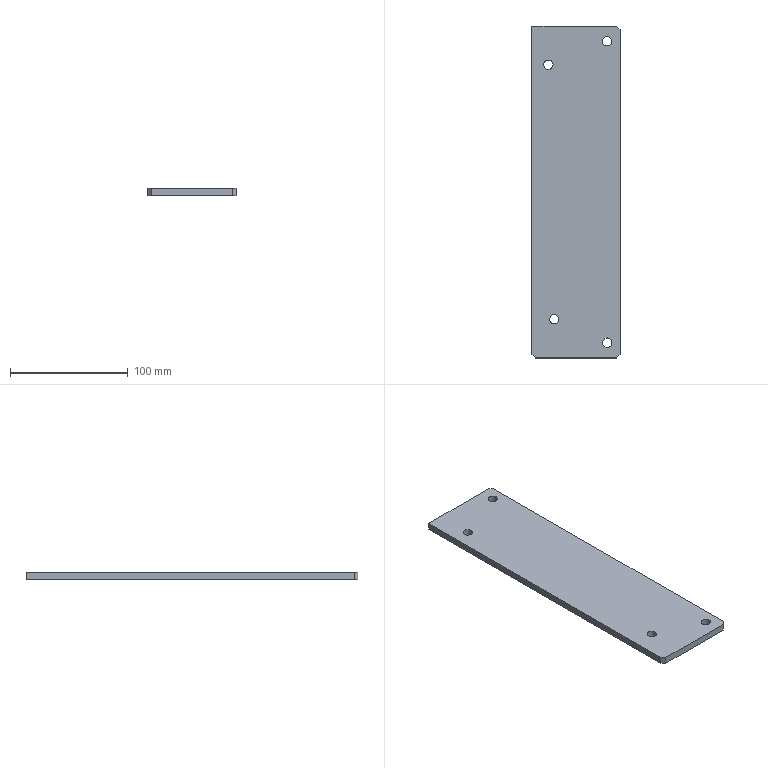Part | STEP file | 1_id1326_x_t | 1 solid | 13 faces | box 75 x 282.347 x 6 mm | volume 125769 mm3 | plane 9 | cylinder 4 | commonest cylinder face diameters 8 x4
STEP:
#1=CARTESIAN_POINT('',(0.,0.,0.));
#2=DIRECTION('',(0.,0.,1.));
#3=DIRECTION('',(1.,0.,0.));
#4=AXIS2_PLACEMENT_3D('',#1,#2,#3);
#5=CARTESIAN_POINT('',(-8.,318.523,-6.));
#6=VERTEX_POINT('',#5);
#7=CARTESIAN_POINT('',(-80.,318.523,-6.));
#8=VERTEX_POINT('',#7);
#9=CARTESIAN_POINT('',(-8.,318.523,-6.));
#10=DIRECTION('',(-1.,0.,0.));
#11=VECTOR('',#10,1.);
#12=LINE('',#9,#11);
#13=CARTESIAN_POINT('',(-80.,-0.15,-6.));
#14=DIRECTION('',(0.,0.,-1.));
#15=DIRECTION('',(-1.,0.,0.));
#16=AXIS2_PLACEMENT_3D('',#13,#14,#15);
#17=PLANE('',#16);
#18=CARTESIAN_POINT('',(-72.,318.673));
#19=DIRECTION('',(1.,0.));
#20=VECTOR('',#19,1.);
#21=LINE('',#18,#20);
#22=(GEOMETRIC_REPRESENTATION_CONTEXT(2)PARAMETRIC_REPRESENTATION_CONTEXT()REPRESENTATION_CONTEXT('',''));
#23=DEFINITIONAL_REPRESENTATION('',(#21),#22);
#24=PCURVE('',#17,#23);
#25=CARTESIAN_POINT('',(669.363,318.523,-130.047));
#26=DIRECTION('',(0.,1.,0.));
#27=DIRECTION('',(-1.,0.,0.));
#28=AXIS2_PLACEMENT_3D('',#25,#26,#27);
#29=PLANE('',#28);
#30=CARTESIAN_POINT('',(677.363,124.047));
#31=DIRECTION('',(1.,0.));
#32=VECTOR('',#31,1.);
#33=LINE('',#30,#32);
#34=(GEOMETRIC_REPRESENTATION_CONTEXT(2)PARAMETRIC_REPRESENTATION_CONTEXT()REPRESENTATION_CONTEXT('',''));
#35=DEFINITIONAL_REPRESENTATION('',(#33),#34);
#36=PCURVE('',#29,#35);
#37=SURFACE_CURVE('',#12,(#24,#36),.PCURVE_S1.);
#38=EDGE_CURVE('',#6,#8,#37,.T.);
#39=ORIENTED_EDGE('',*,*,#38,.F.);
#40=CARTESIAN_POINT('',(-5.,315.523,-6.));
#41=VERTEX_POINT('',#40);
#42=CARTESIAN_POINT('',(-8.,318.523,-6.));
#43=DIRECTION('',(0.7071,-0.7071,0.));
#44=VECTOR('',#43,1.);
#45=LINE('',#42,#44);
#46=CARTESIAN_POINT('',(-72.,318.673));
#47=DIRECTION('',(-0.7071,-0.7071));
#48=VECTOR('',#47,1.);
#49=LINE('',#46,#48);
#50=(GEOMETRIC_REPRESENTATION_CONTEXT(2)PARAMETRIC_REPRESENTATION_CONTEXT()REPRESENTATION_CONTEXT('',''));
#51=DEFINITIONAL_REPRESENTATION('',(#49),#50);
#52=PCURVE('',#17,#51);
#53=CARTESIAN_POINT('',(-8.,318.523,-130.047));
#54=DIRECTION('',(0.7071,0.7071,0.));
#55=DIRECTION('',(-0.7071,0.7071,0.));
#56=AXIS2_PLACEMENT_3D('',#53,#54,#55);
#57=PLANE('',#56);
#58=CARTESIAN_POINT('',(0.,124.047));
#59=DIRECTION('',(-1.,0.));
#60=VECTOR('',#59,1.);
#61=LINE('',#58,#60);
#62=(GEOMETRIC_REPRESENTATION_CONTEXT(2)PARAMETRIC_REPRESENTATION_CONTEXT()REPRESENTATION_CONTEXT('',''));
#63=DEFINITIONAL_REPRESENTATION('',(#61),#62);
#64=PCURVE('',#57,#63);
#65=SURFACE_CURVE('',#45,(#52,#64),.PCURVE_S1.);
#66=EDGE_CURVE('',#6,#41,#65,.T.);
#67=ORIENTED_EDGE('',*,*,#66,.T.);
#68=CARTESIAN_POINT('',(-5.,39.177,-6.));
#69=VERTEX_POINT('',#68);
#70=CARTESIAN_POINT('',(-5.,315.523,-6.));
#71=DIRECTION('',(0.,-1.,0.));
#72=VECTOR('',#71,1.);
#73=LINE('',#70,#72);
#74=CARTESIAN_POINT('',(-75.,315.673));
#75=DIRECTION('',(0.,-1.));
#76=VECTOR('',#75,1.);
#77=LINE('',#74,#76);
#78=(GEOMETRIC_REPRESENTATION_CONTEXT(2)PARAMETRIC_REPRESENTATION_CONTEXT()REPRESENTATION_CONTEXT('',''));
#79=DEFINITIONAL_REPRESENTATION('',(#77),#78);
#80=PCURVE('',#17,#79);
#81=CARTESIAN_POINT('',(-5.,-0.15,0.));
#82=DIRECTION('',(-1.,0.,0.));
#83=DIRECTION('',(0.,-1.,0.));
#84=AXIS2_PLACEMENT_3D('',#81,#82,#83);
#85=PLANE('',#84);
#86=CARTESIAN_POINT('',(-315.673,-6.));
#87=DIRECTION('',(1.,0.));
#88=VECTOR('',#87,1.);
#89=LINE('',#86,#88);
#90=(GEOMETRIC_REPRESENTATION_CONTEXT(2)PARAMETRIC_REPRESENTATION_CONTEXT()REPRESENTATION_CONTEXT('',''));
#91=DEFINITIONAL_REPRESENTATION('',(#89),#90);
#92=PCURVE('',#85,#91);
#93=SURFACE_CURVE('',#73,(#80,#92),.PCURVE_S1.);
#94=EDGE_CURVE('',#41,#69,#93,.T.);
#95=ORIENTED_EDGE('',*,*,#94,.T.);
#96=CARTESIAN_POINT('',(-8.,36.177,-6.));
#97=VERTEX_POINT('',#96);
#98=CARTESIAN_POINT('',(-5.,39.177,-6.));
#99=DIRECTION('',(-0.7071,-0.7071,0.));
#100=VECTOR('',#99,1.);
#101=LINE('',#98,#100);
#102=CARTESIAN_POINT('',(-75.,39.327));
#103=DIRECTION('',(0.7071,-0.7071));
#104=VECTOR('',#103,1.);
#105=LINE('',#102,#104);
#106=(GEOMETRIC_REPRESENTATION_CONTEXT(2)PARAMETRIC_REPRESENTATION_CONTEXT()REPRESENTATION_CONTEXT('',''));
#107=DEFINITIONAL_REPRESENTATION('',(#105),#106);
#108=PCURVE('',#17,#107);
#109=CARTESIAN_POINT('',(-5.,39.177,0.));
#110=DIRECTION('',(0.7071,-0.7071,0.));
#111=DIRECTION('',(0.7071,0.7071,0.));
#112=AXIS2_PLACEMENT_3D('',#109,#110,#111);
#113=PLANE('',#112);
#114=CARTESIAN_POINT('',(0.,-6.));
#115=DIRECTION('',(-1.,0.));
#116=VECTOR('',#115,1.);
#117=LINE('',#114,#116);
#118=(GEOMETRIC_REPRESENTATION_CONTEXT(2)PARAMETRIC_REPRESENTATION_CONTEXT()REPRESENTATION_CONTEXT('',''));
#119=DEFINITIONAL_REPRESENTATION('',(#117),#118);
#120=PCURVE('',#113,#119);
#121=SURFACE_CURVE('',#101,(#108,#120),.PCURVE_S1.);
#122=EDGE_CURVE('',#69,#97,#121,.T.);
#123=ORIENTED_EDGE('',*,*,#122,.T.);
#124=CARTESIAN_POINT('',(-77.,36.177,-6.));
#125=VERTEX_POINT('',#124);
#126=CARTESIAN_POINT('',(-8.,36.177,-6.));
#127=DIRECTION('',(-1.,0.,0.));
#128=VECTOR('',#127,1.);
#129=LINE('',#126,#128);
#130=CARTESIAN_POINT('',(-72.,36.327));
#131=DIRECTION('',(1.,0.));
#132=VECTOR('',#131,1.);
#133=LINE('',#130,#132);
#134=(GEOMETRIC_REPRESENTATION_CONTEXT(2)PARAMETRIC_REPRESENTATION_CONTEXT()REPRESENTATION_CONTEXT('',''));
#135=DEFINITIONAL_REPRESENTATION('',(#133),#134);
#136=PCURVE('',#17,#135);
#137=CARTESIAN_POINT('',(661.363,36.177,-130.047));
#138=DIRECTION('',(0.,-1.,0.));
#139=DIRECTION('',(-1.,0.,0.));
#140=AXIS2_PLACEMENT_3D('',#137,#138,#139);
#141=PLANE('',#140);
#142=CARTESIAN_POINT('',(669.363,-124.047));
#143=DIRECTION('',(1.,0.));
#144=VECTOR('',#143,1.);
#145=LINE('',#142,#144);
#146=(GEOMETRIC_REPRESENTATION_CONTEXT(2)PARAMETRIC_REPRESENTATION_CONTEXT()REPRESENTATION_CONTEXT('',''));
#147=DEFINITIONAL_REPRESENTATION('',(#145),#146);
#148=PCURVE('',#141,#147);
#149=SURFACE_CURVE('',#129,(#136,#148),.PCURVE_S1.);
#150=EDGE_CURVE('',#97,#125,#149,.T.);
#151=ORIENTED_EDGE('',*,*,#150,.T.);
#152=CARTESIAN_POINT('',(-80.,39.177,-6.));
#153=VERTEX_POINT('',#152);
#154=CARTESIAN_POINT('',(-77.,36.177,-6.));
#155=DIRECTION('',(-0.7071,0.7071,0.));
#156=VECTOR('',#155,1.);
#157=LINE('',#154,#156);
#158=CARTESIAN_POINT('',(-3.,36.327));
#159=DIRECTION('',(0.7071,0.7071));
#160=VECTOR('',#159,1.);
#161=LINE('',#158,#160);
#162=(GEOMETRIC_REPRESENTATION_CONTEXT(2)PARAMETRIC_REPRESENTATION_CONTEXT()REPRESENTATION_CONTEXT('',''));
#163=DEFINITIONAL_REPRESENTATION('',(#161),#162);
#164=PCURVE('',#17,#163);
#165=CARTESIAN_POINT('',(-77.,36.177,-130.047));
#166=DIRECTION('',(0.7071,0.7071,0.));
#167=DIRECTION('',(-0.7071,0.7071,0.));
#168=AXIS2_PLACEMENT_3D('',#165,#166,#167);
#169=PLANE('',#168);
#170=CARTESIAN_POINT('',(0.,124.047));
#171=DIRECTION('',(1.,0.));
#172=VECTOR('',#171,1.);
#173=LINE('',#170,#172);
#174=(GEOMETRIC_REPRESENTATION_CONTEXT(2)PARAMETRIC_REPRESENTATION_CONTEXT()REPRESENTATION_CONTEXT('',''));
#175=DEFINITIONAL_REPRESENTATION('',(#173),#174);
#176=PCURVE('',#169,#175);
#177=SURFACE_CURVE('',#157,(#164,#176),.PCURVE_S1.);
#178=EDGE_CURVE('',#125,#153,#177,.T.);
#179=ORIENTED_EDGE('',*,*,#178,.T.);
#180=CARTESIAN_POINT('',(-80.,318.523,-6.));
#181=DIRECTION('',(0.,-1.,0.));
#182=VECTOR('',#181,1.);
#183=LINE('',#180,#182);
#184=CARTESIAN_POINT('',(0.,318.673));
#185=DIRECTION('',(0.,-1.));
#186=VECTOR('',#185,1.);
#187=LINE('',#184,#186);
#188=(GEOMETRIC_REPRESENTATION_CONTEXT(2)PARAMETRIC_REPRESENTATION_CONTEXT()REPRESENTATION_CONTEXT('',''));
#189=DEFINITIONAL_REPRESENTATION('',(#187),#188);
#190=PCURVE('',#17,#189);
#191=CARTESIAN_POINT('',(-80.,-0.15,0.));
#192=DIRECTION('',(-1.,0.,0.));
#193=DIRECTION('',(0.,-1.,0.));
#194=AXIS2_PLACEMENT_3D('',#191,#192,#193);
#195=PLANE('',#194);
#196=CARTESIAN_POINT('',(-318.673,-6.));
#197=DIRECTION('',(1.,0.));
#198=VECTOR('',#197,1.);
#199=LINE('',#196,#198);
#200=(GEOMETRIC_REPRESENTATION_CONTEXT(2)PARAMETRIC_REPRESENTATION_CONTEXT()REPRESENTATION_CONTEXT('',''));
#201=DEFINITIONAL_REPRESENTATION('',(#199),#200);
#202=PCURVE('',#195,#201);
#203=SURFACE_CURVE('',#183,(#190,#202),.PCURVE_S1.);
#204=EDGE_CURVE('',#8,#153,#203,.T.);
#205=ORIENTED_EDGE('',*,*,#204,.F.);
#206=EDGE_LOOP('',(#39,#67,#95,#123,#151,#179,#205));
#207=FACE_BOUND('',#206,.T.);
#208=CARTESIAN_POINT('',(-16.,45.177,-6.));
#209=VERTEX_POINT('',#208);
#210=CARTESIAN_POINT('',(-16.,53.177,-6.));
#211=VERTEX_POINT('',#210);
#212=CARTESIAN_POINT('',(-16.,49.177,-6.));
#213=DIRECTION('',(0.,0.,1.));
#214=DIRECTION('',(0.,-1.,0.));
#215=AXIS2_PLACEMENT_3D('',#212,#213,#214);
#216=CIRCLE('',#215,4.);
#217=CARTESIAN_POINT('',(-64.,45.327));
#218=CARTESIAN_POINT('',(-70.928,45.327));
#219=CARTESIAN_POINT('',(-67.464,51.327));
#220=CARTESIAN_POINT('',(-64.,57.327));
#221=CARTESIAN_POINT('',(-60.536,51.327));
#222=CARTESIAN_POINT('',(-57.072,45.327));
#223=CARTESIAN_POINT('',(-64.,45.327));
#224=(BOUNDED_CURVE()B_SPLINE_CURVE(2,(#217,#218,#219,#220,#221,#222,#223),.UNSPECIFIED.,.T.,.F.)B_SPLINE_CURVE_WITH_KNOTS((1,2,2,2,2,1),(-2.094,0.,2.094,4.189,6.283,8.378),.UNSPECIFIED.)CURVE()GEOMETRIC_REPRESENTATION_ITEM()RATIONAL_B_SPLINE_CURVE((1.,0.5,1.,0.5,1.,0.5,1.))REPRESENTATION_ITEM(''));
#225=(GEOMETRIC_REPRESENTATION_CONTEXT(2)PARAMETRIC_REPRESENTATION_CONTEXT()REPRESENTATION_CONTEXT('',''));
#226=DEFINITIONAL_REPRESENTATION('',(#224),#225);
#227=PCURVE('',#17,#226);
#228=CARTESIAN_POINT('',(-16.,49.177,-6.));
#229=DIRECTION('',(0.,0.,1.));
#230=DIRECTION('',(0.,1.,0.));
#231=AXIS2_PLACEMENT_3D('',#228,#229,#230);
#232=CYLINDRICAL_SURFACE('',#231,4.);
#233=CARTESIAN_POINT('',(3.142,0.));
#234=DIRECTION('',(1.,0.));
#235=VECTOR('',#234,1.);
#236=LINE('',#233,#235);
#237=(GEOMETRIC_REPRESENTATION_CONTEXT(2)PARAMETRIC_REPRESENTATION_CONTEXT()REPRESENTATION_CONTEXT('',''));
#238=DEFINITIONAL_REPRESENTATION('',(#236),#237);
#239=PCURVE('',#232,#238);
#240=SURFACE_CURVE('',#216,(#227,#239),.PCURVE_S1.);
#241=EDGE_CURVE('',#209,#211,#240,.T.);
#242=ORIENTED_EDGE('',*,*,#241,.T.);
#243=CARTESIAN_POINT('',(-16.,49.177,-6.));
#244=DIRECTION('',(0.,0.,1.));
#245=DIRECTION('',(0.,-1.,0.));
#246=AXIS2_PLACEMENT_3D('',#243,#244,#245);
#247=CIRCLE('',#246,4.);
#248=CARTESIAN_POINT('',(-64.,45.327));
#249=CARTESIAN_POINT('',(-70.928,45.327));
#250=CARTESIAN_POINT('',(-67.464,51.327));
#251=CARTESIAN_POINT('',(-64.,57.327));
#252=CARTESIAN_POINT('',(-60.536,51.327));
#253=CARTESIAN_POINT('',(-57.072,45.327));
#254=CARTESIAN_POINT('',(-64.,45.327));
#255=(BOUNDED_CURVE()B_SPLINE_CURVE(2,(#248,#249,#250,#251,#252,#253,#254),.UNSPECIFIED.,.T.,.F.)B_SPLINE_CURVE_WITH_KNOTS((1,2,2,2,2,1),(-2.094,0.,2.094,4.189,6.283,8.378),.UNSPECIFIED.)CURVE()GEOMETRIC_REPRESENTATION_ITEM()RATIONAL_B_SPLINE_CURVE((1.,0.5,1.,0.5,1.,0.5,1.))REPRESENTATION_ITEM(''));
#256=(GEOMETRIC_REPRESENTATION_CONTEXT(2)PARAMETRIC_REPRESENTATION_CONTEXT()REPRESENTATION_CONTEXT('',''));
#257=DEFINITIONAL_REPRESENTATION('',(#255),#256);
#258=PCURVE('',#17,#257);
#259=CARTESIAN_POINT('',(-3.142,0.));
#260=DIRECTION('',(1.,0.));
#261=VECTOR('',#260,1.);
#262=LINE('',#259,#261);
#263=(GEOMETRIC_REPRESENTATION_CONTEXT(2)PARAMETRIC_REPRESENTATION_CONTEXT()REPRESENTATION_CONTEXT('',''));
#264=DEFINITIONAL_REPRESENTATION('',(#262),#263);
#265=PCURVE('',#232,#264);
#266=SURFACE_CURVE('',#247,(#258,#265),.PCURVE_S1.);
#267=EDGE_CURVE('',#211,#209,#266,.T.);
#268=ORIENTED_EDGE('',*,*,#267,.T.);
#269=EDGE_LOOP('',(#242,#268));
#270=FACE_BOUND('',#269,.T.);
#271=CARTESIAN_POINT('',(-61.,65.177,-6.));
#272=VERTEX_POINT('',#271);
#273=CARTESIAN_POINT('',(-57.,69.177,-6.));
#274=VERTEX_POINT('',#273);
#275=CARTESIAN_POINT('',(-61.,69.177,-6.));
#276=DIRECTION('',(0.,0.,1.));
#277=DIRECTION('',(0.,-1.,0.));
#278=AXIS2_PLACEMENT_3D('',#275,#276,#277);
#279=CIRCLE('',#278,4.);
#280=CARTESIAN_POINT('',(-19.,65.327));
#281=CARTESIAN_POINT('',(-25.928,65.327));
#282=CARTESIAN_POINT('',(-22.464,71.327));
#283=CARTESIAN_POINT('',(-19.,77.327));
#284=CARTESIAN_POINT('',(-15.536,71.327));
#285=CARTESIAN_POINT('',(-12.072,65.327));
#286=CARTESIAN_POINT('',(-19.,65.327));
#287=(BOUNDED_CURVE()B_SPLINE_CURVE(2,(#280,#281,#282,#283,#284,#285,#286),.UNSPECIFIED.,.T.,.F.)B_SPLINE_CURVE_WITH_KNOTS((1,2,2,2,2,1),(-2.094,0.,2.094,4.189,6.283,8.378),.UNSPECIFIED.)CURVE()GEOMETRIC_REPRESENTATION_ITEM()RATIONAL_B_SPLINE_CURVE((1.,0.5,1.,0.5,1.,0.5,1.))REPRESENTATION_ITEM(''));
#288=(GEOMETRIC_REPRESENTATION_CONTEXT(2)PARAMETRIC_REPRESENTATION_CONTEXT()REPRESENTATION_CONTEXT('',''));
#289=DEFINITIONAL_REPRESENTATION('',(#287),#288);
#290=PCURVE('',#17,#289);
#291=CARTESIAN_POINT('',(-61.,69.177,-6.));
#292=DIRECTION('',(0.,0.,1.));
#293=DIRECTION('',(0.,1.,0.));
#294=AXIS2_PLACEMENT_3D('',#291,#292,#293);
#295=CYLINDRICAL_SURFACE('',#294,4.);
#296=CARTESIAN_POINT('',(9.425,0.));
#297=DIRECTION('',(1.,0.));
#298=VECTOR('',#297,1.);
#299=LINE('',#296,#298);
#300=(GEOMETRIC_REPRESENTATION_CONTEXT(2)PARAMETRIC_REPRESENTATION_CONTEXT()REPRESENTATION_CONTEXT('',''));
#301=DEFINITIONAL_REPRESENTATION('',(#299),#300);
#302=PCURVE('',#295,#301);
#303=SURFACE_CURVE('',#279,(#290,#302),.PCURVE_S1.);
#304=EDGE_CURVE('',#272,#274,#303,.T.);
#305=ORIENTED_EDGE('',*,*,#304,.T.);
#306=CARTESIAN_POINT('',(-61.,69.177,-6.));
#307=DIRECTION('',(0.,0.,1.));
#308=DIRECTION('',(0.,-1.,0.));
#309=AXIS2_PLACEMENT_3D('',#306,#307,#308);
#310=CIRCLE('',#309,4.);
#311=CARTESIAN_POINT('',(-19.,65.327));
#312=CARTESIAN_POINT('',(-25.928,65.327));
#313=CARTESIAN_POINT('',(-22.464,71.327));
#314=CARTESIAN_POINT('',(-19.,77.327));
#315=CARTESIAN_POINT('',(-15.536,71.327));
#316=CARTESIAN_POINT('',(-12.072,65.327));
#317=CARTESIAN_POINT('',(-19.,65.327));
#318=(BOUNDED_CURVE()B_SPLINE_CURVE(2,(#311,#312,#313,#314,#315,#316,#317),.UNSPECIFIED.,.T.,.F.)B_SPLINE_CURVE_WITH_KNOTS((1,2,2,2,2,1),(-2.094,0.,2.094,4.189,6.283,8.378),.UNSPECIFIED.)CURVE()GEOMETRIC_REPRESENTATION_ITEM()RATIONAL_B_SPLINE_CURVE((1.,0.5,1.,0.5,1.,0.5,1.))REPRESENTATION_ITEM(''));
#319=(GEOMETRIC_REPRESENTATION_CONTEXT(2)PARAMETRIC_REPRESENTATION_CONTEXT()REPRESENTATION_CONTEXT('',''));
#320=DEFINITIONAL_REPRESENTATION('',(#318),#319);
#321=PCURVE('',#17,#320);
#322=CARTESIAN_POINT('',(3.142,0.));
#323=DIRECTION('',(1.,0.));
#324=VECTOR('',#323,1.);
#325=LINE('',#322,#324);
#326=(GEOMETRIC_REPRESENTATION_CONTEXT(2)PARAMETRIC_REPRESENTATION_CONTEXT()REPRESENTATION_CONTEXT('',''));
#327=DEFINITIONAL_REPRESENTATION('',(#325),#326);
#328=PCURVE('',#295,#327);
#329=SURFACE_CURVE('',#310,(#321,#328),.PCURVE_S1.);
#330=EDGE_CURVE('',#274,#272,#329,.T.);
#331=ORIENTED_EDGE('',*,*,#330,.T.);
#332=EDGE_LOOP('',(#305,#331));
#333=FACE_BOUND('',#332,.T.);
#334=CARTESIAN_POINT('',(-66.,289.523,-6.));
#335=VERTEX_POINT('',#334);
#336=CARTESIAN_POINT('',(-62.,285.523,-6.));
#337=VERTEX_POINT('',#336);
#338=CARTESIAN_POINT('',(-66.,285.523,-6.));
#339=DIRECTION('',(0.,0.,1.));
#340=DIRECTION('',(0.,1.,0.));
#341=AXIS2_PLACEMENT_3D('',#338,#339,#340);
#342=CIRCLE('',#341,4.);
#343=CARTESIAN_POINT('',(-14.,289.673));
#344=CARTESIAN_POINT('',(-7.072,289.673));
#345=CARTESIAN_POINT('',(-10.536,283.673));
#346=CARTESIAN_POINT('',(-14.,277.673));
#347=CARTESIAN_POINT('',(-17.464,283.673));
#348=CARTESIAN_POINT('',(-20.928,289.673));
#349=CARTESIAN_POINT('',(-14.,289.673));
#350=(BOUNDED_CURVE()B_SPLINE_CURVE(2,(#343,#344,#345,#346,#347,#348,#349),.UNSPECIFIED.,.T.,.F.)B_SPLINE_CURVE_WITH_KNOTS((1,2,2,2,2,1),(-2.094,0.,2.094,4.189,6.283,8.378),.UNSPECIFIED.)CURVE()GEOMETRIC_REPRESENTATION_ITEM()RATIONAL_B_SPLINE_CURVE((1.,0.5,1.,0.5,1.,0.5,1.))REPRESENTATION_ITEM(''));
#351=(GEOMETRIC_REPRESENTATION_CONTEXT(2)PARAMETRIC_REPRESENTATION_CONTEXT()REPRESENTATION_CONTEXT('',''));
#352=DEFINITIONAL_REPRESENTATION('',(#350),#351);
#353=PCURVE('',#17,#352);
#354=CARTESIAN_POINT('',(-66.,285.523,-6.));
#355=DIRECTION('',(0.,0.,1.));
#356=DIRECTION('',(0.,-1.,0.));
#357=AXIS2_PLACEMENT_3D('',#354,#355,#356);
#358=CYLINDRICAL_SURFACE('',#357,4.);
#359=CARTESIAN_POINT('',(3.142,0.));
#360=DIRECTION('',(1.,0.));
#361=VECTOR('',#360,1.);
#362=LINE('',#359,#361);
#363=(GEOMETRIC_REPRESENTATION_CONTEXT(2)PARAMETRIC_REPRESENTATION_CONTEXT()REPRESENTATION_CONTEXT('',''));
#364=DEFINITIONAL_REPRESENTATION('',(#362),#363);
#365=PCURVE('',#358,#364);
#366=SURFACE_CURVE('',#342,(#353,#365),.PCURVE_S1.);
#367=EDGE_CURVE('',#335,#337,#366,.T.);
#368=ORIENTED_EDGE('',*,*,#367,.T.);
#369=CARTESIAN_POINT('',(-66.,285.523,-6.));
#370=DIRECTION('',(0.,0.,1.));
#371=DIRECTION('',(0.,1.,0.));
#372=AXIS2_PLACEMENT_3D('',#369,#370,#371);
#373=CIRCLE('',#372,4.);
#374=CARTESIAN_POINT('',(-14.,289.673));
#375=CARTESIAN_POINT('',(-7.072,289.673));
#376=CARTESIAN_POINT('',(-10.536,283.673));
#377=CARTESIAN_POINT('',(-14.,277.673));
#378=CARTESIAN_POINT('',(-17.464,283.673));
#379=CARTESIAN_POINT('',(-20.928,289.673));
#380=CARTESIAN_POINT('',(-14.,289.673));
#381=(BOUNDED_CURVE()B_SPLINE_CURVE(2,(#374,#375,#376,#377,#378,#379,#380),.UNSPECIFIED.,.T.,.F.)B_SPLINE_CURVE_WITH_KNOTS((1,2,2,2,2,1),(-2.094,0.,2.094,4.189,6.283,8.378),.UNSPECIFIED.)CURVE()GEOMETRIC_REPRESENTATION_ITEM()RATIONAL_B_SPLINE_CURVE((1.,0.5,1.,0.5,1.,0.5,1.))REPRESENTATION_ITEM(''));
#382=(GEOMETRIC_REPRESENTATION_CONTEXT(2)PARAMETRIC_REPRESENTATION_CONTEXT()REPRESENTATION_CONTEXT('',''));
#383=DEFINITIONAL_REPRESENTATION('',(#381),#382);
#384=PCURVE('',#17,#383);
#385=CARTESIAN_POINT('',(-3.142,0.));
#386=DIRECTION('',(1.,0.));
#387=VECTOR('',#386,1.);
#388=LINE('',#385,#387);
#389=(GEOMETRIC_REPRESENTATION_CONTEXT(2)PARAMETRIC_REPRESENTATION_CONTEXT()REPRESENTATION_CONTEXT('',''));
#390=DEFINITIONAL_REPRESENTATION('',(#388),#389);
#391=PCURVE('',#358,#390);
#392=SURFACE_CURVE('',#373,(#384,#391),.PCURVE_S1.);
#393=EDGE_CURVE('',#337,#335,#392,.T.);
#394=ORIENTED_EDGE('',*,*,#393,.T.);
#395=EDGE_LOOP('',(#368,#394));
#396=FACE_BOUND('',#395,.T.);
#397=CARTESIAN_POINT('',(-16.,309.523,-6.));
#398=VERTEX_POINT('',#397);
#399=CARTESIAN_POINT('',(-12.,305.523,-6.));
#400=VERTEX_POINT('',#399);
#401=CARTESIAN_POINT('',(-16.,305.523,-6.));
#402=DIRECTION('',(0.,0.,1.));
#403=DIRECTION('',(0.,1.,0.));
#404=AXIS2_PLACEMENT_3D('',#401,#402,#403);
#405=CIRCLE('',#404,4.);
#406=CARTESIAN_POINT('',(-64.,309.673));
#407=CARTESIAN_POINT('',(-57.072,309.673));
#408=CARTESIAN_POINT('',(-60.536,303.673));
#409=CARTESIAN_POINT('',(-64.,297.673));
#410=CARTESIAN_POINT('',(-67.464,303.673));
#411=CARTESIAN_POINT('',(-70.928,309.673));
#412=CARTESIAN_POINT('',(-64.,309.673));
#413=(BOUNDED_CURVE()B_SPLINE_CURVE(2,(#406,#407,#408,#409,#410,#411,#412),.UNSPECIFIED.,.T.,.F.)B_SPLINE_CURVE_WITH_KNOTS((1,2,2,2,2,1),(-2.094,0.,2.094,4.189,6.283,8.378),.UNSPECIFIED.)CURVE()GEOMETRIC_REPRESENTATION_ITEM()RATIONAL_B_SPLINE_CURVE((1.,0.5,1.,0.5,1.,0.5,1.))REPRESENTATION_ITEM(''));
#414=(GEOMETRIC_REPRESENTATION_CONTEXT(2)PARAMETRIC_REPRESENTATION_CONTEXT()REPRESENTATION_CONTEXT('',''));
#415=DEFINITIONAL_REPRESENTATION('',(#413),#414);
#416=PCURVE('',#17,#415);
#417=CARTESIAN_POINT('',(-16.,305.523,-6.));
#418=DIRECTION('',(0.,0.,1.));
#419=DIRECTION('',(0.,-1.,0.));
#420=AXIS2_PLACEMENT_3D('',#417,#418,#419);
#421=CYLINDRICAL_SURFACE('',#420,4.);
#422=CARTESIAN_POINT('',(3.142,0.));
#423=DIRECTION('',(1.,0.));
#424=VECTOR('',#423,1.);
#425=LINE('',#422,#424);
#426=(GEOMETRIC_REPRESENTATION_CONTEXT(2)PARAMETRIC_REPRESENTATION_CONTEXT()REPRESENTATION_CONTEXT('',''));
#427=DEFINITIONAL_REPRESENTATION('',(#425),#426);
#428=PCURVE('',#421,#427);
#429=SURFACE_CURVE('',#405,(#416,#428),.PCURVE_S1.);
#430=EDGE_CURVE('',#398,#400,#429,.T.);
#431=ORIENTED_EDGE('',*,*,#430,.T.);
#432=CARTESIAN_POINT('',(-16.,305.523,-6.));
#433=DIRECTION('',(0.,0.,1.));
#434=DIRECTION('',(0.,1.,0.));
#435=AXIS2_PLACEMENT_3D('',#432,#433,#434);
#436=CIRCLE('',#435,4.);
#437=CARTESIAN_POINT('',(-64.,309.673));
#438=CARTESIAN_POINT('',(-57.072,309.673));
#439=CARTESIAN_POINT('',(-60.536,303.673));
#440=CARTESIAN_POINT('',(-64.,297.673));
#441=CARTESIAN_POINT('',(-67.464,303.673));
#442=CARTESIAN_POINT('',(-70.928,309.673));
#443=CARTESIAN_POINT('',(-64.,309.673));
#444=(BOUNDED_CURVE()B_SPLINE_CURVE(2,(#437,#438,#439,#440,#441,#442,#443),.UNSPECIFIED.,.T.,.F.)B_SPLINE_CURVE_WITH_KNOTS((1,2,2,2,2,1),(-2.094,0.,2.094,4.189,6.283,8.378),.UNSPECIFIED.)CURVE()GEOMETRIC_REPRESENTATION_ITEM()RATIONAL_B_SPLINE_CURVE((1.,0.5,1.,0.5,1.,0.5,1.))REPRESENTATION_ITEM(''));
#445=(GEOMETRIC_REPRESENTATION_CONTEXT(2)PARAMETRIC_REPRESENTATION_CONTEXT()REPRESENTATION_CONTEXT('',''));
#446=DEFINITIONAL_REPRESENTATION('',(#444),#445);
#447=PCURVE('',#17,#446);
#448=CARTESIAN_POINT('',(-3.142,0.));
#449=DIRECTION('',(1.,0.));
#450=VECTOR('',#449,1.);
#451=LINE('',#448,#450);
#452=(GEOMETRIC_REPRESENTATION_CONTEXT(2)PARAMETRIC_REPRESENTATION_CONTEXT()REPRESENTATION_CONTEXT('',''));
#453=DEFINITIONAL_REPRESENTATION('',(#451),#452);
#454=PCURVE('',#421,#453);
#455=SURFACE_CURVE('',#436,(#447,#454),.PCURVE_S1.);
#456=EDGE_CURVE('',#400,#398,#455,.T.);
#457=ORIENTED_EDGE('',*,*,#456,.T.);
#458=EDGE_LOOP('',(#431,#457));
#459=FACE_BOUND('',#458,.T.);
#460=ADVANCED_FACE('',(#207,#270,#333,#396,#459),#17,.T.);
#461=CARTESIAN_POINT('',(-16.,53.177,0.));
#462=VERTEX_POINT('',#461);
#463=CARTESIAN_POINT('',(-16.,49.177,0.));
#464=DIRECTION('',(0.,0.,-1.));
#465=DIRECTION('',(0.,1.,0.));
#466=AXIS2_PLACEMENT_3D('',#463,#464,#465);
#467=CIRCLE('',#466,4.);
#468=CARTESIAN_POINT('',(6.283,6.));
#469=DIRECTION('',(-1.,0.));
#470=VECTOR('',#469,1.);
#471=LINE('',#468,#470);
#472=(GEOMETRIC_REPRESENTATION_CONTEXT(2)PARAMETRIC_REPRESENTATION_CONTEXT()REPRESENTATION_CONTEXT('',''));
#473=DEFINITIONAL_REPRESENTATION('',(#471),#472);
#474=PCURVE('',#232,#473);
#475=CARTESIAN_POINT('',(-80.,-0.15,0.));
#476=DIRECTION('',(0.,0.,-1.));
#477=DIRECTION('',(-1.,0.,0.));
#478=AXIS2_PLACEMENT_3D('',#475,#476,#477);
#479=PLANE('',#478);
#480=CARTESIAN_POINT('',(-64.,49.327));
#481=DIRECTION('',(0.,1.));
#482=AXIS2_PLACEMENT_2D('',#480,#481);
#483=CIRCLE('',#482,4.);
#484=(GEOMETRIC_REPRESENTATION_CONTEXT(2)PARAMETRIC_REPRESENTATION_CONTEXT()REPRESENTATION_CONTEXT('',''));
#485=DEFINITIONAL_REPRESENTATION('',(#483),#484);
#486=PCURVE('',#479,#485);
#487=SURFACE_CURVE('',#467,(#474,#486),.PCURVE_S1.);
#488=EDGE_CURVE('',#462,#462,#487,.T.);
#489=ORIENTED_EDGE('',*,*,#488,.T.);
#490=CARTESIAN_POINT('',(-16.,53.177,-6.));
#491=CARTESIAN_POINT('',(-16.,53.177,0.));
#492=B_SPLINE_CURVE_WITH_KNOTS('',1,(#490,#491),.UNSPECIFIED.,.F.,.F.,(2,2),(0.,6.),.PIECEWISE_BEZIER_KNOTS.);
#493=CARTESIAN_POINT('',(0.,0.));
#494=DIRECTION('',(0.,1.));
#495=VECTOR('',#494,1.);
#496=LINE('',#493,#495);
#497=(GEOMETRIC_REPRESENTATION_CONTEXT(2)PARAMETRIC_REPRESENTATION_CONTEXT()REPRESENTATION_CONTEXT('',''));
#498=DEFINITIONAL_REPRESENTATION('',(#496),#497);
#499=PCURVE('',#232,#498);
#500=CARTESIAN_POINT('',(6.283,0.));
#501=DIRECTION('',(0.,1.));
#502=VECTOR('',#501,1.);
#503=LINE('',#500,#502);
#504=(GEOMETRIC_REPRESENTATION_CONTEXT(2)PARAMETRIC_REPRESENTATION_CONTEXT()REPRESENTATION_CONTEXT('',''));
#505=DEFINITIONAL_REPRESENTATION('',(#503),#504);
#506=PCURVE('',#232,#505);
#507=SEAM_CURVE('',#492,(#499,#506),.PCURVE_S1.);
#508=EDGE_CURVE('',#211,#462,#507,.T.);
#509=ORIENTED_EDGE('',*,*,#508,.F.);
#510=ORIENTED_EDGE('',*,*,#267,.T.);
#511=ORIENTED_EDGE('',*,*,#241,.T.);
#512=ORIENTED_EDGE('',*,*,#508,.T.);
#513=EDGE_LOOP('',(#489,#509,#510,#511,#512));
#514=FACE_BOUND('',#513,.F.);
#515=ADVANCED_FACE('',(#514),#232,.F.);
#516=CARTESIAN_POINT('',(-5.,315.523,0.));
#517=VERTEX_POINT('',#516);
#518=CARTESIAN_POINT('',(-8.,318.523,0.));
#519=VERTEX_POINT('',#518);
#520=CARTESIAN_POINT('',(-5.,315.523,0.));
#521=DIRECTION('',(-0.7071,0.7071,0.));
#522=VECTOR('',#521,1.);
#523=LINE('',#520,#522);
#524=CARTESIAN_POINT('',(-75.,315.673));
#525=DIRECTION('',(0.7071,0.7071));
#526=VECTOR('',#525,1.);
#527=LINE('',#524,#526);
#528=(GEOMETRIC_REPRESENTATION_CONTEXT(2)PARAMETRIC_REPRESENTATION_CONTEXT()REPRESENTATION_CONTEXT('',''));
#529=DEFINITIONAL_REPRESENTATION('',(#527),#528);
#530=PCURVE('',#479,#529);
#531=CARTESIAN_POINT('',(-4.243,130.047));
#532=DIRECTION('',(1.,0.));
#533=VECTOR('',#532,1.);
#534=LINE('',#531,#533);
#535=(GEOMETRIC_REPRESENTATION_CONTEXT(2)PARAMETRIC_REPRESENTATION_CONTEXT()REPRESENTATION_CONTEXT('',''));
#536=DEFINITIONAL_REPRESENTATION('',(#534),#535);
#537=PCURVE('',#57,#536);
#538=SURFACE_CURVE('',#523,(#530,#537),.PCURVE_S1.);
#539=EDGE_CURVE('',#517,#519,#538,.T.);
#540=ORIENTED_EDGE('',*,*,#539,.T.);
#541=CARTESIAN_POINT('',(-80.,318.523,0.));
#542=VERTEX_POINT('',#541);
#543=CARTESIAN_POINT('',(-8.,318.523,0.));
#544=DIRECTION('',(-1.,0.,0.));
#545=VECTOR('',#544,1.);
#546=LINE('',#543,#545);
#547=CARTESIAN_POINT('',(-72.,318.673));
#548=DIRECTION('',(1.,0.));
#549=VECTOR('',#548,1.);
#550=LINE('',#547,#549);
#551=(GEOMETRIC_REPRESENTATION_CONTEXT(2)PARAMETRIC_REPRESENTATION_CONTEXT()REPRESENTATION_CONTEXT('',''));
#552=DEFINITIONAL_REPRESENTATION('',(#550),#551);
#553=PCURVE('',#479,#552);
#554=CARTESIAN_POINT('',(677.363,130.047));
#555=DIRECTION('',(1.,0.));
#556=VECTOR('',#555,1.);
#557=LINE('',#554,#556);
#558=(GEOMETRIC_REPRESENTATION_CONTEXT(2)PARAMETRIC_REPRESENTATION_CONTEXT()REPRESENTATION_CONTEXT('',''));
#559=DEFINITIONAL_REPRESENTATION('',(#557),#558);
#560=PCURVE('',#29,#559);
#561=SURFACE_CURVE('',#546,(#553,#560),.PCURVE_S1.);
#562=EDGE_CURVE('',#519,#542,#561,.T.);
#563=ORIENTED_EDGE('',*,*,#562,.T.);
#564=CARTESIAN_POINT('',(-80.,39.177,0.));
#565=VERTEX_POINT('',#564);
#566=CARTESIAN_POINT('',(-80.,318.523,0.));
#567=DIRECTION('',(0.,-1.,0.));
#568=VECTOR('',#567,1.);
#569=LINE('',#566,#568);
#570=CARTESIAN_POINT('',(0.,318.673));
#571=DIRECTION('',(0.,-1.));
#572=VECTOR('',#571,1.);
#573=LINE('',#570,#572);
#574=(GEOMETRIC_REPRESENTATION_CONTEXT(2)PARAMETRIC_REPRESENTATION_CONTEXT()REPRESENTATION_CONTEXT('',''));
#575=DEFINITIONAL_REPRESENTATION('',(#573),#574);
#576=PCURVE('',#479,#575);
#577=CARTESIAN_POINT('',(-318.673,0.));
#578=DIRECTION('',(1.,0.));
#579=VECTOR('',#578,1.);
#580=LINE('',#577,#579);
#581=(GEOMETRIC_REPRESENTATION_CONTEXT(2)PARAMETRIC_REPRESENTATION_CONTEXT()REPRESENTATION_CONTEXT('',''));
#582=DEFINITIONAL_REPRESENTATION('',(#580),#581);
#583=PCURVE('',#195,#582);
#584=SURFACE_CURVE('',#569,(#576,#583),.PCURVE_S1.);
#585=EDGE_CURVE('',#542,#565,#584,.T.);
#586=ORIENTED_EDGE('',*,*,#585,.T.);
#587=CARTESIAN_POINT('',(-77.,36.177,0.));
#588=VERTEX_POINT('',#587);
#589=CARTESIAN_POINT('',(-80.,39.177,0.));
#590=DIRECTION('',(0.7071,-0.7071,0.));
#591=VECTOR('',#590,1.);
#592=LINE('',#589,#591);
#593=CARTESIAN_POINT('',(0.,39.327));
#594=DIRECTION('',(-0.7071,-0.7071));
#595=VECTOR('',#594,1.);
#596=LINE('',#593,#595);
#597=(GEOMETRIC_REPRESENTATION_CONTEXT(2)PARAMETRIC_REPRESENTATION_CONTEXT()REPRESENTATION_CONTEXT('',''));
#598=DEFINITIONAL_REPRESENTATION('',(#596),#597);
#599=PCURVE('',#479,#598);
#600=CARTESIAN_POINT('',(4.243,130.047));
#601=DIRECTION('',(-1.,0.));
#602=VECTOR('',#601,1.);
#603=LINE('',#600,#602);
#604=(GEOMETRIC_REPRESENTATION_CONTEXT(2)PARAMETRIC_REPRESENTATION_CONTEXT()REPRESENTATION_CONTEXT('',''));
#605=DEFINITIONAL_REPRESENTATION('',(#603),#604);
#606=PCURVE('',#169,#605);
#607=SURFACE_CURVE('',#592,(#599,#606),.PCURVE_S1.);
#608=EDGE_CURVE('',#565,#588,#607,.T.);
#609=ORIENTED_EDGE('',*,*,#608,.T.);
#610=CARTESIAN_POINT('',(-8.,36.177,0.));
#611=VERTEX_POINT('',#610);
#612=CARTESIAN_POINT('',(-8.,36.177,0.));
#613=DIRECTION('',(-1.,0.,0.));
#614=VECTOR('',#613,1.);
#615=LINE('',#612,#614);
#616=CARTESIAN_POINT('',(-72.,36.327));
#617=DIRECTION('',(1.,0.));
#618=VECTOR('',#617,1.);
#619=LINE('',#616,#618);
#620=(GEOMETRIC_REPRESENTATION_CONTEXT(2)PARAMETRIC_REPRESENTATION_CONTEXT()REPRESENTATION_CONTEXT('',''));
#621=DEFINITIONAL_REPRESENTATION('',(#619),#620);
#622=PCURVE('',#479,#621);
#623=CARTESIAN_POINT('',(669.363,-130.047));
#624=DIRECTION('',(1.,0.));
#625=VECTOR('',#624,1.);
#626=LINE('',#623,#625);
#627=(GEOMETRIC_REPRESENTATION_CONTEXT(2)PARAMETRIC_REPRESENTATION_CONTEXT()REPRESENTATION_CONTEXT('',''));
#628=DEFINITIONAL_REPRESENTATION('',(#626),#627);
#629=PCURVE('',#141,#628);
#630=SURFACE_CURVE('',#615,(#622,#629),.PCURVE_S1.);
#631=EDGE_CURVE('',#611,#588,#630,.T.);
#632=ORIENTED_EDGE('',*,*,#631,.F.);
#633=CARTESIAN_POINT('',(-5.,39.177,0.));
#634=VERTEX_POINT('',#633);
#635=CARTESIAN_POINT('',(-8.,36.177,0.));
#636=DIRECTION('',(0.7071,0.7071,0.));
#637=VECTOR('',#636,1.);
#638=LINE('',#635,#637);
#639=CARTESIAN_POINT('',(-72.,36.327));
#640=DIRECTION('',(-0.7071,0.7071));
#641=VECTOR('',#640,1.);
#642=LINE('',#639,#641);
#643=(GEOMETRIC_REPRESENTATION_CONTEXT(2)PARAMETRIC_REPRESENTATION_CONTEXT()REPRESENTATION_CONTEXT('',''));
#644=DEFINITIONAL_REPRESENTATION('',(#642),#643);
#645=PCURVE('',#479,#644);
#646=CARTESIAN_POINT('',(-4.243,0.));
#647=DIRECTION('',(1.,0.));
#648=VECTOR('',#647,1.);
#649=LINE('',#646,#648);
#650=(GEOMETRIC_REPRESENTATION_CONTEXT(2)PARAMETRIC_REPRESENTATION_CONTEXT()REPRESENTATION_CONTEXT('',''));
#651=DEFINITIONAL_REPRESENTATION('',(#649),#650);
#652=PCURVE('',#113,#651);
#653=SURFACE_CURVE('',#638,(#645,#652),.PCURVE_S1.);
#654=EDGE_CURVE('',#611,#634,#653,.T.);
#655=ORIENTED_EDGE('',*,*,#654,.T.);
#656=CARTESIAN_POINT('',(-5.,315.523,0.));
#657=DIRECTION('',(0.,-1.,0.));
#658=VECTOR('',#657,1.);
#659=LINE('',#656,#658);
#660=CARTESIAN_POINT('',(-75.,315.673));
#661=DIRECTION('',(0.,-1.));
#662=VECTOR('',#661,1.);
#663=LINE('',#660,#662);
#664=(GEOMETRIC_REPRESENTATION_CONTEXT(2)PARAMETRIC_REPRESENTATION_CONTEXT()REPRESENTATION_CONTEXT('',''));
#665=DEFINITIONAL_REPRESENTATION('',(#663),#664);
#666=PCURVE('',#479,#665);
#667=CARTESIAN_POINT('',(-315.673,0.));
#668=DIRECTION('',(1.,0.));
#669=VECTOR('',#668,1.);
#670=LINE('',#667,#669);
#671=(GEOMETRIC_REPRESENTATION_CONTEXT(2)PARAMETRIC_REPRESENTATION_CONTEXT()REPRESENTATION_CONTEXT('',''));
#672=DEFINITIONAL_REPRESENTATION('',(#670),#671);
#673=PCURVE('',#85,#672);
#674=SURFACE_CURVE('',#659,(#666,#673),.PCURVE_S1.);
#675=EDGE_CURVE('',#517,#634,#674,.T.);
#676=ORIENTED_EDGE('',*,*,#675,.F.);
#677=EDGE_LOOP('',(#540,#563,#586,#609,#632,#655,#676));
#678=FACE_BOUND('',#677,.T.);
#679=ORIENTED_EDGE('',*,*,#488,.T.);
#680=EDGE_LOOP('',(#679));
#681=FACE_BOUND('',#680,.T.);
#682=CARTESIAN_POINT('',(-57.,69.177,0.));
#683=VERTEX_POINT('',#682);
#684=CARTESIAN_POINT('',(-61.,69.177,0.));
#685=DIRECTION('',(0.,0.,-1.));
#686=DIRECTION('',(1.,0.,0.));
#687=AXIS2_PLACEMENT_3D('',#684,#685,#686);
#688=CIRCLE('',#687,4.);
#689=CARTESIAN_POINT('',(-19.,69.327));
#690=DIRECTION('',(-1.,0.));
#691=AXIS2_PLACEMENT_2D('',#689,#690);
#692=CIRCLE('',#691,4.);
#693=(GEOMETRIC_REPRESENTATION_CONTEXT(2)PARAMETRIC_REPRESENTATION_CONTEXT()REPRESENTATION_CONTEXT('',''));
#694=DEFINITIONAL_REPRESENTATION('',(#692),#693);
#695=PCURVE('',#479,#694);
#696=CARTESIAN_POINT('',(10.996,6.));
#697=DIRECTION('',(-1.,0.));
#698=VECTOR('',#697,1.);
#699=LINE('',#696,#698);
#700=(GEOMETRIC_REPRESENTATION_CONTEXT(2)PARAMETRIC_REPRESENTATION_CONTEXT()REPRESENTATION_CONTEXT('',''));
#701=DEFINITIONAL_REPRESENTATION('',(#699),#700);
#702=PCURVE('',#295,#701);
#703=SURFACE_CURVE('',#688,(#695,#702),.PCURVE_S1.);
#704=EDGE_CURVE('',#683,#683,#703,.T.);
#705=ORIENTED_EDGE('',*,*,#704,.T.);
#706=EDGE_LOOP('',(#705));
#707=FACE_BOUND('',#706,.T.);
#708=CARTESIAN_POINT('',(-12.,305.523,0.));
#709=VERTEX_POINT('',#708);
#710=CARTESIAN_POINT('',(-16.,305.523,0.));
#711=DIRECTION('',(0.,0.,-1.));
#712=DIRECTION('',(1.,0.,0.));
#713=AXIS2_PLACEMENT_3D('',#710,#711,#712);
#714=CIRCLE('',#713,4.);
#715=CARTESIAN_POINT('',(-64.,305.673));
#716=DIRECTION('',(-1.,0.));
#717=AXIS2_PLACEMENT_2D('',#715,#716);
#718=CIRCLE('',#717,4.);
#719=(GEOMETRIC_REPRESENTATION_CONTEXT(2)PARAMETRIC_REPRESENTATION_CONTEXT()REPRESENTATION_CONTEXT('',''));
#720=DEFINITIONAL_REPRESENTATION('',(#718),#719);
#721=PCURVE('',#479,#720);
#722=CARTESIAN_POINT('',(7.854,6.));
#723=DIRECTION('',(-1.,0.));
#724=VECTOR('',#723,1.);
#725=LINE('',#722,#724);
#726=(GEOMETRIC_REPRESENTATION_CONTEXT(2)PARAMETRIC_REPRESENTATION_CONTEXT()REPRESENTATION_CONTEXT('',''));
#727=DEFINITIONAL_REPRESENTATION('',(#725),#726);
#728=PCURVE('',#421,#727);
#729=SURFACE_CURVE('',#714,(#721,#728),.PCURVE_S1.);
#730=EDGE_CURVE('',#709,#709,#729,.T.);
#731=ORIENTED_EDGE('',*,*,#730,.T.);
#732=EDGE_LOOP('',(#731));
#733=FACE_BOUND('',#732,.T.);
#734=CARTESIAN_POINT('',(-62.,285.523,0.));
#735=VERTEX_POINT('',#734);
#736=CARTESIAN_POINT('',(-66.,285.523,0.));
#737=DIRECTION('',(0.,0.,-1.));
#738=DIRECTION('',(1.,0.,0.));
#739=AXIS2_PLACEMENT_3D('',#736,#737,#738);
#740=CIRCLE('',#739,4.);
#741=CARTESIAN_POINT('',(-14.,285.673));
#742=DIRECTION('',(-1.,0.));
#743=AXIS2_PLACEMENT_2D('',#741,#742);
#744=CIRCLE('',#743,4.);
#745=(GEOMETRIC_REPRESENTATION_CONTEXT(2)PARAMETRIC_REPRESENTATION_CONTEXT()REPRESENTATION_CONTEXT('',''));
#746=DEFINITIONAL_REPRESENTATION('',(#744),#745);
#747=PCURVE('',#479,#746);
#748=CARTESIAN_POINT('',(7.854,6.));
#749=DIRECTION('',(-1.,0.));
#750=VECTOR('',#749,1.);
#751=LINE('',#748,#750);
#752=(GEOMETRIC_REPRESENTATION_CONTEXT(2)PARAMETRIC_REPRESENTATION_CONTEXT()REPRESENTATION_CONTEXT('',''));
#753=DEFINITIONAL_REPRESENTATION('',(#751),#752);
#754=PCURVE('',#358,#753);
#755=SURFACE_CURVE('',#740,(#747,#754),.PCURVE_S1.);
#756=EDGE_CURVE('',#735,#735,#755,.T.);
#757=ORIENTED_EDGE('',*,*,#756,.T.);
#758=EDGE_LOOP('',(#757));
#759=FACE_BOUND('',#758,.T.);
#760=ADVANCED_FACE('',(#678,#681,#707,#733,#759),#479,.F.);
#761=ORIENTED_EDGE('',*,*,#704,.T.);
#762=CARTESIAN_POINT('',(-57.,69.177,-6.));
#763=CARTESIAN_POINT('',(-57.,69.177,0.));
#764=B_SPLINE_CURVE_WITH_KNOTS('',1,(#762,#763),.UNSPECIFIED.,.F.,.F.,(2,2),(0.,6.),.PIECEWISE_BEZIER_KNOTS.);
#765=CARTESIAN_POINT('',(4.712,0.));
#766=DIRECTION('',(0.,1.));
#767=VECTOR('',#766,1.);
#768=LINE('',#765,#767);
#769=(GEOMETRIC_REPRESENTATION_CONTEXT(2)PARAMETRIC_REPRESENTATION_CONTEXT()REPRESENTATION_CONTEXT('',''));
#770=DEFINITIONAL_REPRESENTATION('',(#768),#769);
#771=PCURVE('',#295,#770);
#772=CARTESIAN_POINT('',(10.996,0.));
#773=DIRECTION('',(0.,1.));
#774=VECTOR('',#773,1.);
#775=LINE('',#772,#774);
#776=(GEOMETRIC_REPRESENTATION_CONTEXT(2)PARAMETRIC_REPRESENTATION_CONTEXT()REPRESENTATION_CONTEXT('',''));
#777=DEFINITIONAL_REPRESENTATION('',(#775),#776);
#778=PCURVE('',#295,#777);
#779=SEAM_CURVE('',#764,(#771,#778),.PCURVE_S1.);
#780=EDGE_CURVE('',#274,#683,#779,.T.);
#781=ORIENTED_EDGE('',*,*,#780,.F.);
#782=ORIENTED_EDGE('',*,*,#330,.T.);
#783=ORIENTED_EDGE('',*,*,#304,.T.);
#784=ORIENTED_EDGE('',*,*,#780,.T.);
#785=EDGE_LOOP('',(#761,#781,#782,#783,#784));
#786=FACE_BOUND('',#785,.F.);
#787=ADVANCED_FACE('',(#786),#295,.F.);
#788=CARTESIAN_POINT('',(-5.,315.523,0.));
#789=DIRECTION('',(0.,0.,-1.));
#790=VECTOR('',#789,1.);
#791=LINE('',#788,#790);
#792=CARTESIAN_POINT('',(-315.673,0.));
#793=DIRECTION('',(0.,-1.));
#794=VECTOR('',#793,1.);
#795=LINE('',#792,#794);
#796=(GEOMETRIC_REPRESENTATION_CONTEXT(2)PARAMETRIC_REPRESENTATION_CONTEXT()REPRESENTATION_CONTEXT('',''));
#797=DEFINITIONAL_REPRESENTATION('',(#795),#796);
#798=PCURVE('',#85,#797);
#799=CARTESIAN_POINT('',(-4.243,130.047));
#800=DIRECTION('',(0.,-1.));
#801=VECTOR('',#800,1.);
#802=LINE('',#799,#801);
#803=(GEOMETRIC_REPRESENTATION_CONTEXT(2)PARAMETRIC_REPRESENTATION_CONTEXT()REPRESENTATION_CONTEXT('',''));
#804=DEFINITIONAL_REPRESENTATION('',(#802),#803);
#805=PCURVE('',#57,#804);
#806=SURFACE_CURVE('',#791,(#798,#805),.PCURVE_S1.);
#807=EDGE_CURVE('',#517,#41,#806,.T.);
#808=ORIENTED_EDGE('',*,*,#807,.F.);
#809=ORIENTED_EDGE('',*,*,#675,.T.);
#810=CARTESIAN_POINT('',(-5.,39.177,-6.));
#811=DIRECTION('',(0.,0.,1.));
#812=VECTOR('',#811,1.);
#813=LINE('',#810,#812);
#814=CARTESIAN_POINT('',(-39.327,-6.));
#815=DIRECTION('',(0.,1.));
#816=VECTOR('',#815,1.);
#817=LINE('',#814,#816);
#818=(GEOMETRIC_REPRESENTATION_CONTEXT(2)PARAMETRIC_REPRESENTATION_CONTEXT()REPRESENTATION_CONTEXT('',''));
#819=DEFINITIONAL_REPRESENTATION('',(#817),#818);
#820=PCURVE('',#85,#819);
#821=CARTESIAN_POINT('',(0.,-6.));
#822=DIRECTION('',(0.,1.));
#823=VECTOR('',#822,1.);
#824=LINE('',#821,#823);
#825=(GEOMETRIC_REPRESENTATION_CONTEXT(2)PARAMETRIC_REPRESENTATION_CONTEXT()REPRESENTATION_CONTEXT('',''));
#826=DEFINITIONAL_REPRESENTATION('',(#824),#825);
#827=PCURVE('',#113,#826);
#828=SURFACE_CURVE('',#813,(#820,#827),.PCURVE_S1.);
#829=EDGE_CURVE('',#69,#634,#828,.T.);
#830=ORIENTED_EDGE('',*,*,#829,.F.);
#831=ORIENTED_EDGE('',*,*,#94,.F.);
#832=EDGE_LOOP('',(#808,#809,#830,#831));
#833=FACE_BOUND('',#832,.T.);
#834=ADVANCED_FACE('',(#833),#85,.F.);
#835=CARTESIAN_POINT('',(-8.,36.177,0.));
#836=DIRECTION('',(0.,0.,-1.));
#837=VECTOR('',#836,1.);
#838=LINE('',#835,#837);
#839=CARTESIAN_POINT('',(-4.243,0.));
#840=DIRECTION('',(0.,-1.));
#841=VECTOR('',#840,1.);
#842=LINE('',#839,#841);
#843=(GEOMETRIC_REPRESENTATION_CONTEXT(2)PARAMETRIC_REPRESENTATION_CONTEXT()REPRESENTATION_CONTEXT('',''));
#844=DEFINITIONAL_REPRESENTATION('',(#842),#843);
#845=PCURVE('',#113,#844);
#846=CARTESIAN_POINT('',(669.363,-130.047));
#847=DIRECTION('',(0.,1.));
#848=VECTOR('',#847,1.);
#849=LINE('',#846,#848);
#850=(GEOMETRIC_REPRESENTATION_CONTEXT(2)PARAMETRIC_REPRESENTATION_CONTEXT()REPRESENTATION_CONTEXT('',''));
#851=DEFINITIONAL_REPRESENTATION('',(#849),#850);
#852=PCURVE('',#141,#851);
#853=SURFACE_CURVE('',#838,(#845,#852),.PCURVE_S1.);
#854=EDGE_CURVE('',#611,#97,#853,.T.);
#855=ORIENTED_EDGE('',*,*,#854,.T.);
#856=ORIENTED_EDGE('',*,*,#122,.F.);
#857=ORIENTED_EDGE('',*,*,#829,.T.);
#858=ORIENTED_EDGE('',*,*,#654,.F.);
#859=EDGE_LOOP('',(#855,#856,#857,#858));
#860=FACE_BOUND('',#859,.T.);
#861=ADVANCED_FACE('',(#860),#113,.T.);
#862=CARTESIAN_POINT('',(-77.,36.177,-6.));
#863=DIRECTION('',(0.,0.,1.));
#864=VECTOR('',#863,1.);
#865=LINE('',#862,#864);
#866=CARTESIAN_POINT('',(738.363,-124.047));
#867=DIRECTION('',(0.,-1.));
#868=VECTOR('',#867,1.);
#869=LINE('',#866,#868);
#870=(GEOMETRIC_REPRESENTATION_CONTEXT(2)PARAMETRIC_REPRESENTATION_CONTEXT()REPRESENTATION_CONTEXT('',''));
#871=DEFINITIONAL_REPRESENTATION('',(#869),#870);
#872=PCURVE('',#141,#871);
#873=CARTESIAN_POINT('',(0.,124.047));
#874=DIRECTION('',(0.,1.));
#875=VECTOR('',#874,1.);
#876=LINE('',#873,#875);
#877=(GEOMETRIC_REPRESENTATION_CONTEXT(2)PARAMETRIC_REPRESENTATION_CONTEXT()REPRESENTATION_CONTEXT('',''));
#878=DEFINITIONAL_REPRESENTATION('',(#876),#877);
#879=PCURVE('',#169,#878);
#880=SURFACE_CURVE('',#865,(#872,#879),.PCURVE_S1.);
#881=EDGE_CURVE('',#125,#588,#880,.T.);
#882=ORIENTED_EDGE('',*,*,#881,.F.);
#883=ORIENTED_EDGE('',*,*,#150,.F.);
#884=ORIENTED_EDGE('',*,*,#854,.F.);
#885=ORIENTED_EDGE('',*,*,#631,.T.);
#886=EDGE_LOOP('',(#882,#883,#884,#885));
#887=FACE_BOUND('',#886,.T.);
#888=ADVANCED_FACE('',(#887),#141,.T.);
#889=CARTESIAN_POINT('',(-80.,39.177,0.));
#890=DIRECTION('',(0.,0.,-1.));
#891=VECTOR('',#890,1.);
#892=LINE('',#889,#891);
#893=CARTESIAN_POINT('',(4.243,130.047));
#894=DIRECTION('',(0.,-1.));
#895=VECTOR('',#894,1.);
#896=LINE('',#893,#895);
#897=(GEOMETRIC_REPRESENTATION_CONTEXT(2)PARAMETRIC_REPRESENTATION_CONTEXT()REPRESENTATION_CONTEXT('',''));
#898=DEFINITIONAL_REPRESENTATION('',(#896),#897);
#899=PCURVE('',#169,#898);
#900=CARTESIAN_POINT('',(-39.327,0.));
#901=DIRECTION('',(0.,-1.));
#902=VECTOR('',#901,1.);
#903=LINE('',#900,#902);
#904=(GEOMETRIC_REPRESENTATION_CONTEXT(2)PARAMETRIC_REPRESENTATION_CONTEXT()REPRESENTATION_CONTEXT('',''));
#905=DEFINITIONAL_REPRESENTATION('',(#903),#904);
#906=PCURVE('',#195,#905);
#907=SURFACE_CURVE('',#892,(#899,#906),.PCURVE_S1.);
#908=EDGE_CURVE('',#565,#153,#907,.T.);
#909=ORIENTED_EDGE('',*,*,#908,.T.);
#910=ORIENTED_EDGE('',*,*,#178,.F.);
#911=ORIENTED_EDGE('',*,*,#881,.T.);
#912=ORIENTED_EDGE('',*,*,#608,.F.);
#913=EDGE_LOOP('',(#909,#910,#911,#912));
#914=FACE_BOUND('',#913,.T.);
#915=ADVANCED_FACE('',(#914),#169,.F.);
#916=CARTESIAN_POINT('',(-80.,318.523,0.));
#917=DIRECTION('',(0.,0.,-1.));
#918=VECTOR('',#917,1.);
#919=LINE('',#916,#918);
#920=CARTESIAN_POINT('',(-318.673,0.));
#921=DIRECTION('',(0.,-1.));
#922=VECTOR('',#921,1.);
#923=LINE('',#920,#922);
#924=(GEOMETRIC_REPRESENTATION_CONTEXT(2)PARAMETRIC_REPRESENTATION_CONTEXT()REPRESENTATION_CONTEXT('',''));
#925=DEFINITIONAL_REPRESENTATION('',(#923),#924);
#926=PCURVE('',#195,#925);
#927=CARTESIAN_POINT('',(749.363,130.047));
#928=DIRECTION('',(0.,-1.));
#929=VECTOR('',#928,1.);
#930=LINE('',#927,#929);
#931=(GEOMETRIC_REPRESENTATION_CONTEXT(2)PARAMETRIC_REPRESENTATION_CONTEXT()REPRESENTATION_CONTEXT('',''));
#932=DEFINITIONAL_REPRESENTATION('',(#930),#931);
#933=PCURVE('',#29,#932);
#934=SURFACE_CURVE('',#919,(#926,#933),.PCURVE_S1.);
#935=EDGE_CURVE('',#542,#8,#934,.T.);
#936=ORIENTED_EDGE('',*,*,#935,.T.);
#937=ORIENTED_EDGE('',*,*,#204,.T.);
#938=ORIENTED_EDGE('',*,*,#908,.F.);
#939=ORIENTED_EDGE('',*,*,#585,.F.);
#940=EDGE_LOOP('',(#936,#937,#938,#939));
#941=FACE_BOUND('',#940,.T.);
#942=ADVANCED_FACE('',(#941),#195,.T.);
#943=CARTESIAN_POINT('',(-8.,318.523,-6.));
#944=DIRECTION('',(0.,0.,1.));
#945=VECTOR('',#944,1.);
#946=LINE('',#943,#945);
#947=CARTESIAN_POINT('',(677.363,124.047));
#948=DIRECTION('',(0.,1.));
#949=VECTOR('',#948,1.);
#950=LINE('',#947,#949);
#951=(GEOMETRIC_REPRESENTATION_CONTEXT(2)PARAMETRIC_REPRESENTATION_CONTEXT()REPRESENTATION_CONTEXT('',''));
#952=DEFINITIONAL_REPRESENTATION('',(#950),#951);
#953=PCURVE('',#29,#952);
#954=CARTESIAN_POINT('',(0.,124.047));
#955=DIRECTION('',(0.,1.));
#956=VECTOR('',#955,1.);
#957=LINE('',#954,#956);
#958=(GEOMETRIC_REPRESENTATION_CONTEXT(2)PARAMETRIC_REPRESENTATION_CONTEXT()REPRESENTATION_CONTEXT('',''));
#959=DEFINITIONAL_REPRESENTATION('',(#957),#958);
#960=PCURVE('',#57,#959);
#961=SURFACE_CURVE('',#946,(#953,#960),.PCURVE_S1.);
#962=EDGE_CURVE('',#6,#519,#961,.T.);
#963=ORIENTED_EDGE('',*,*,#962,.F.);
#964=ORIENTED_EDGE('',*,*,#38,.T.);
#965=ORIENTED_EDGE('',*,*,#935,.F.);
#966=ORIENTED_EDGE('',*,*,#562,.F.);
#967=EDGE_LOOP('',(#963,#964,#965,#966));
#968=FACE_BOUND('',#967,.T.);
#969=ADVANCED_FACE('',(#968),#29,.T.);
#970=ORIENTED_EDGE('',*,*,#807,.T.);
#971=ORIENTED_EDGE('',*,*,#66,.F.);
#972=ORIENTED_EDGE('',*,*,#962,.T.);
#973=ORIENTED_EDGE('',*,*,#539,.F.);
#974=EDGE_LOOP('',(#970,#971,#972,#973));
#975=FACE_BOUND('',#974,.T.);
#976=ADVANCED_FACE('',(#975),#57,.T.);
#977=ORIENTED_EDGE('',*,*,#730,.T.);
#978=CARTESIAN_POINT('',(-12.,305.523,-6.));
#979=CARTESIAN_POINT('',(-12.,305.523,0.));
#980=B_SPLINE_CURVE_WITH_KNOTS('',1,(#978,#979),.UNSPECIFIED.,.F.,.F.,(2,2),(0.,6.),.PIECEWISE_BEZIER_KNOTS.);
#981=CARTESIAN_POINT('',(1.571,0.));
#982=DIRECTION('',(0.,1.));
#983=VECTOR('',#982,1.);
#984=LINE('',#981,#983);
#985=(GEOMETRIC_REPRESENTATION_CONTEXT(2)PARAMETRIC_REPRESENTATION_CONTEXT()REPRESENTATION_CONTEXT('',''));
#986=DEFINITIONAL_REPRESENTATION('',(#984),#985);
#987=PCURVE('',#421,#986);
#988=CARTESIAN_POINT('',(7.854,0.));
#989=DIRECTION('',(0.,1.));
#990=VECTOR('',#989,1.);
#991=LINE('',#988,#990);
#992=(GEOMETRIC_REPRESENTATION_CONTEXT(2)PARAMETRIC_REPRESENTATION_CONTEXT()REPRESENTATION_CONTEXT('',''));
#993=DEFINITIONAL_REPRESENTATION('',(#991),#992);
#994=PCURVE('',#421,#993);
#995=SEAM_CURVE('',#980,(#987,#994),.PCURVE_S1.);
#996=EDGE_CURVE('',#400,#709,#995,.T.);
#997=ORIENTED_EDGE('',*,*,#996,.F.);
#998=ORIENTED_EDGE('',*,*,#456,.T.);
#999=ORIENTED_EDGE('',*,*,#430,.T.);
#1000=ORIENTED_EDGE('',*,*,#996,.T.);
#1001=EDGE_LOOP('',(#977,#997,#998,#999,#1000));
#1002=FACE_BOUND('',#1001,.F.);
#1003=ADVANCED_FACE('',(#1002),#421,.F.);
#1004=ORIENTED_EDGE('',*,*,#756,.T.);
#1005=CARTESIAN_POINT('',(-62.,285.523,-6.));
#1006=CARTESIAN_POINT('',(-62.,285.523,0.));
#1007=B_SPLINE_CURVE_WITH_KNOTS('',1,(#1005,#1006),.UNSPECIFIED.,.F.,.F.,(2,2),(0.,6.),.PIECEWISE_BEZIER_KNOTS.);
#1008=CARTESIAN_POINT('',(1.571,0.));
#1009=DIRECTION('',(0.,1.));
#1010=VECTOR('',#1009,1.);
#1011=LINE('',#1008,#1010);
#1012=(GEOMETRIC_REPRESENTATION_CONTEXT(2)PARAMETRIC_REPRESENTATION_CONTEXT()REPRESENTATION_CONTEXT('',''));
#1013=DEFINITIONAL_REPRESENTATION('',(#1011),#1012);
#1014=PCURVE('',#358,#1013);
#1015=CARTESIAN_POINT('',(7.854,0.));
#1016=DIRECTION('',(0.,1.));
#1017=VECTOR('',#1016,1.);
#1018=LINE('',#1015,#1017);
#1019=(GEOMETRIC_REPRESENTATION_CONTEXT(2)PARAMETRIC_REPRESENTATION_CONTEXT()REPRESENTATION_CONTEXT('',''));
#1020=DEFINITIONAL_REPRESENTATION('',(#1018),#1019);
#1021=PCURVE('',#358,#1020);
#1022=SEAM_CURVE('',#1007,(#1014,#1021),.PCURVE_S1.);
#1023=EDGE_CURVE('',#337,#735,#1022,.T.);
#1024=ORIENTED_EDGE('',*,*,#1023,.F.);
#1025=ORIENTED_EDGE('',*,*,#393,.T.);
#1026=ORIENTED_EDGE('',*,*,#367,.T.);
#1027=ORIENTED_EDGE('',*,*,#1023,.T.);
#1028=EDGE_LOOP('',(#1004,#1024,#1025,#1026,#1027));
#1029=FACE_BOUND('',#1028,.F.);
#1030=ADVANCED_FACE('',(#1029),#358,.F.);
#1031=CLOSED_SHELL('',(#460,#515,#760,#787,#834,#861,#888,#915,#942,#969,#976,#1003,#1030));
#1032=MANIFOLD_SOLID_BREP('',#1031);
#1033=(LENGTH_UNIT()NAMED_UNIT(*)SI_UNIT(.MILLI.,.METRE.));
#1034=UNCERTAINTY_MEASURE_WITH_UNIT(LENGTH_MEASURE(0.000002),#1033,'','');
#1035=(NAMED_UNIT(*)PLANE_ANGLE_UNIT()SI_UNIT($,.RADIAN.));
#1036=(NAMED_UNIT(*)SI_UNIT($,.STERADIAN.)SOLID_ANGLE_UNIT());
#1037=(GEOMETRIC_REPRESENTATION_CONTEXT(3)GLOBAL_UNCERTAINTY_ASSIGNED_CONTEXT((#1034))GLOBAL_UNIT_ASSIGNED_CONTEXT((#1033,#1035,#1036))REPRESENTATION_CONTEXT('',''));
#1038=ADVANCED_BREP_SHAPE_REPRESENTATION('',(#4,#1032),#1037);